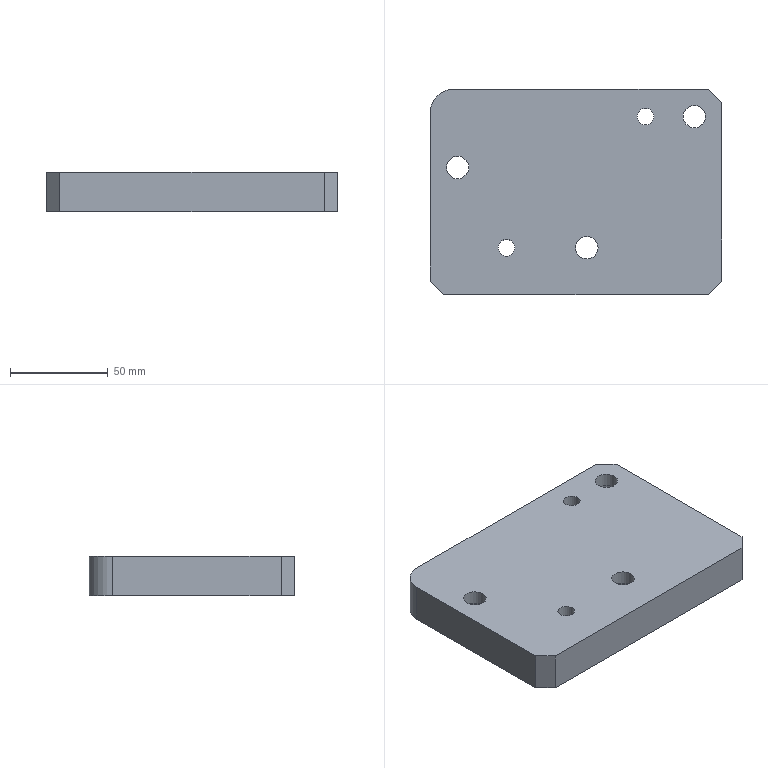Part | STEP file | lll_id606_x_t | 1 solid | 21 faces | box 149 x 105 x 20 mm | volume 296423 mm3 | plane 12 | cylinder 9 | commonest cylinder face diameters 11.509 x3 18.007 x3 8.505 x2 24 x1
STEP:
#1=CARTESIAN_POINT('',(372.248,164.5,2.5));
#2=VERTEX_POINT('',#1);
#3=CARTESIAN_POINT('',(376.5,164.5,2.5));
#4=DIRECTION('',(0.,0.,-1.));
#5=DIRECTION('',(-1.,0.,0.));
#6=AXIS2_PLACEMENT_3D('',#3,#4,#5);
#7=CIRCLE('',#6,4.253);
#8=EDGE_CURVE('',#2,#2,#7,.T.);
#9=ORIENTED_EDGE('',*,*,#8,.F.);
#10=EDGE_LOOP('',(#9));
#11=FACE_BOUND('',#10,.T.);
#12=CARTESIAN_POINT('',(289.504,138.5,2.5));
#13=VERTEX_POINT('',#12);
#14=CARTESIAN_POINT('',(280.5,138.5,2.5));
#15=DIRECTION('',(0.,0.,1.));
#16=DIRECTION('',(1.,0.,0.));
#17=AXIS2_PLACEMENT_3D('',#14,#15,#16);
#18=CIRCLE('',#17,9.004);
#19=EDGE_CURVE('',#13,#13,#18,.T.);
#20=ORIENTED_EDGE('',*,*,#19,.T.);
#21=EDGE_LOOP('',(#20));
#22=FACE_BOUND('',#21,.T.);
#23=CARTESIAN_POINT('',(266.5,166.5,2.5));
#24=VERTEX_POINT('',#23);
#25=CARTESIAN_POINT('',(266.5,80.5,2.5));
#26=VERTEX_POINT('',#25);
#27=CARTESIAN_POINT('',(266.5,130.75,2.5));
#28=DIRECTION('',(0.,-1.,0.));
#29=VECTOR('',#28,1.);
#30=LINE('',#27,#29);
#31=EDGE_CURVE('',#24,#26,#30,.T.);
#32=ORIENTED_EDGE('',*,*,#31,.F.);
#33=CARTESIAN_POINT('',(278.5,178.5,2.5));
#34=VERTEX_POINT('',#33);
#35=CARTESIAN_POINT('',(278.5,166.5,2.5));
#36=DIRECTION('',(0.,0.,-1.));
#37=DIRECTION('',(-1.,0.,0.));
#38=AXIS2_PLACEMENT_3D('',#35,#36,#37);
#39=CIRCLE('',#38,12.);
#40=EDGE_CURVE('',#24,#34,#39,.T.);
#41=ORIENTED_EDGE('',*,*,#40,.T.);
#42=CARTESIAN_POINT('',(408.5,178.5,2.5));
#43=VERTEX_POINT('',#42);
#44=CARTESIAN_POINT('',(437.,178.5,2.5));
#45=DIRECTION('',(-1.,0.,0.));
#46=VECTOR('',#45,1.);
#47=LINE('',#44,#46);
#48=EDGE_CURVE('',#43,#34,#47,.T.);
#49=ORIENTED_EDGE('',*,*,#48,.F.);
#50=CARTESIAN_POINT('',(415.5,171.5,2.5));
#51=VERTEX_POINT('',#50);
#52=CARTESIAN_POINT('',(366.125,220.875,2.5));
#53=DIRECTION('',(-0.7071,0.7071,0.));
#54=VECTOR('',#53,1.);
#55=LINE('',#52,#54);
#56=EDGE_CURVE('',#51,#43,#55,.T.);
#57=ORIENTED_EDGE('',*,*,#56,.F.);
#58=CARTESIAN_POINT('',(415.5,80.5,2.5));
#59=VERTEX_POINT('',#58);
#60=CARTESIAN_POINT('',(415.5,130.75,2.5));
#61=DIRECTION('',(0.,1.,0.));
#62=VECTOR('',#61,1.);
#63=LINE('',#60,#62);
#64=EDGE_CURVE('',#59,#51,#63,.T.);
#65=ORIENTED_EDGE('',*,*,#64,.F.);
#66=CARTESIAN_POINT('',(408.5,73.5,2.5));
#67=VERTEX_POINT('',#66);
#68=CARTESIAN_POINT('',(531.875,196.875,2.5));
#69=DIRECTION('',(0.7071,0.7071,0.));
#70=VECTOR('',#69,1.);
#71=LINE('',#68,#70);
#72=EDGE_CURVE('',#67,#59,#71,.T.);
#73=ORIENTED_EDGE('',*,*,#72,.F.);
#74=CARTESIAN_POINT('',(273.5,73.5,2.5));
#75=VERTEX_POINT('',#74);
#76=CARTESIAN_POINT('',(437.,73.5,2.5));
#77=DIRECTION('',(1.,0.,0.));
#78=VECTOR('',#77,1.);
#79=LINE('',#76,#78);
#80=EDGE_CURVE('',#75,#67,#79,.T.);
#81=ORIENTED_EDGE('',*,*,#80,.F.);
#82=CARTESIAN_POINT('',(246.125,100.875,2.5));
#83=DIRECTION('',(0.7071,-0.7071,0.));
#84=VECTOR('',#83,1.);
#85=LINE('',#82,#84);
#86=EDGE_CURVE('',#26,#75,#85,.T.);
#87=ORIENTED_EDGE('',*,*,#86,.F.);
#88=EDGE_LOOP('',(#32,#41,#49,#57,#65,#73,#81,#87));
#89=FACE_BOUND('',#88,.T.);
#90=CARTESIAN_POINT('',(355.504,97.5,2.5));
#91=VERTEX_POINT('',#90);
#92=CARTESIAN_POINT('',(346.5,97.5,2.5));
#93=DIRECTION('',(0.,0.,1.));
#94=DIRECTION('',(1.,0.,0.));
#95=AXIS2_PLACEMENT_3D('',#92,#93,#94);
#96=CIRCLE('',#95,9.004);
#97=EDGE_CURVE('',#91,#91,#96,.T.);
#98=ORIENTED_EDGE('',*,*,#97,.T.);
#99=EDGE_LOOP('',(#98));
#100=FACE_BOUND('',#99,.T.);
#101=CARTESIAN_POINT('',(301.248,97.5,2.5));
#102=VERTEX_POINT('',#101);
#103=CARTESIAN_POINT('',(305.5,97.5,2.5));
#104=DIRECTION('',(0.,0.,-1.));
#105=DIRECTION('',(-1.,0.,0.));
#106=AXIS2_PLACEMENT_3D('',#103,#104,#105);
#107=CIRCLE('',#106,4.253);
#108=EDGE_CURVE('',#102,#102,#107,.T.);
#109=ORIENTED_EDGE('',*,*,#108,.F.);
#110=EDGE_LOOP('',(#109));
#111=FACE_BOUND('',#110,.T.);
#112=CARTESIAN_POINT('',(410.504,164.5,2.5));
#113=VERTEX_POINT('',#112);
#114=CARTESIAN_POINT('',(401.5,164.5,2.5));
#115=DIRECTION('',(0.,0.,1.));
#116=DIRECTION('',(1.,0.,0.));
#117=AXIS2_PLACEMENT_3D('',#114,#115,#116);
#118=CIRCLE('',#117,9.004);
#119=EDGE_CURVE('',#113,#113,#118,.T.);
#120=ORIENTED_EDGE('',*,*,#119,.T.);
#121=EDGE_LOOP('',(#120));
#122=FACE_BOUND('',#121,.T.);
#123=CARTESIAN_POINT('',(437.,291.75,2.5));
#124=DIRECTION('',(0.,0.,-1.));
#125=DIRECTION('',(1.,0.,0.));
#126=AXIS2_PLACEMENT_3D('',#123,#124,#125);
#127=PLANE('',#126);
#128=ADVANCED_FACE('',(#11,#22,#89,#100,#111,#122),#127,.T.);
#129=CARTESIAN_POINT('',(380.753,164.5,22.5));
#130=VERTEX_POINT('',#129);
#131=CARTESIAN_POINT('',(376.5,164.5,22.5));
#132=DIRECTION('',(0.,0.,1.));
#133=DIRECTION('',(1.,0.,0.));
#134=AXIS2_PLACEMENT_3D('',#131,#132,#133);
#135=CIRCLE('',#134,4.253);
#136=EDGE_CURVE('',#130,#130,#135,.T.);
#137=ORIENTED_EDGE('',*,*,#136,.F.);
#138=EDGE_LOOP('',(#137));
#139=FACE_BOUND('',#138,.T.);
#140=CARTESIAN_POINT('',(407.255,164.5,22.5));
#141=VERTEX_POINT('',#140);
#142=CARTESIAN_POINT('',(401.5,164.5,22.5));
#143=DIRECTION('',(0.,0.,1.));
#144=DIRECTION('',(1.,0.,0.));
#145=AXIS2_PLACEMENT_3D('',#142,#143,#144);
#146=CIRCLE('',#145,5.755);
#147=EDGE_CURVE('',#141,#141,#146,.T.);
#148=ORIENTED_EDGE('',*,*,#147,.F.);
#149=EDGE_LOOP('',(#148));
#150=FACE_BOUND('',#149,.T.);
#151=CARTESIAN_POINT('',(309.753,97.5,22.5));
#152=VERTEX_POINT('',#151);
#153=CARTESIAN_POINT('',(305.5,97.5,22.5));
#154=DIRECTION('',(0.,0.,1.));
#155=DIRECTION('',(1.,0.,0.));
#156=AXIS2_PLACEMENT_3D('',#153,#154,#155);
#157=CIRCLE('',#156,4.253);
#158=EDGE_CURVE('',#152,#152,#157,.T.);
#159=ORIENTED_EDGE('',*,*,#158,.F.);
#160=EDGE_LOOP('',(#159));
#161=FACE_BOUND('',#160,.T.);
#162=CARTESIAN_POINT('',(286.255,138.5,22.5));
#163=VERTEX_POINT('',#162);
#164=CARTESIAN_POINT('',(280.5,138.5,22.5));
#165=DIRECTION('',(0.,0.,1.));
#166=DIRECTION('',(1.,0.,0.));
#167=AXIS2_PLACEMENT_3D('',#164,#165,#166);
#168=CIRCLE('',#167,5.755);
#169=EDGE_CURVE('',#163,#163,#168,.T.);
#170=ORIENTED_EDGE('',*,*,#169,.F.);
#171=EDGE_LOOP('',(#170));
#172=FACE_BOUND('',#171,.T.);
#173=CARTESIAN_POINT('',(352.255,97.5,22.5));
#174=VERTEX_POINT('',#173);
#175=CARTESIAN_POINT('',(346.5,97.5,22.5));
#176=DIRECTION('',(0.,0.,1.));
#177=DIRECTION('',(1.,0.,0.));
#178=AXIS2_PLACEMENT_3D('',#175,#176,#177);
#179=CIRCLE('',#178,5.755);
#180=EDGE_CURVE('',#174,#174,#179,.T.);
#181=ORIENTED_EDGE('',*,*,#180,.F.);
#182=EDGE_LOOP('',(#181));
#183=FACE_BOUND('',#182,.T.);
#184=CARTESIAN_POINT('',(278.5,178.5,22.5));
#185=VERTEX_POINT('',#184);
#186=CARTESIAN_POINT('',(408.5,178.5,22.5));
#187=VERTEX_POINT('',#186);
#188=CARTESIAN_POINT('',(437.,178.5,22.5));
#189=DIRECTION('',(1.,0.,0.));
#190=VECTOR('',#189,1.);
#191=LINE('',#188,#190);
#192=EDGE_CURVE('',#185,#187,#191,.T.);
#193=ORIENTED_EDGE('',*,*,#192,.F.);
#194=CARTESIAN_POINT('',(266.5,166.5,22.5));
#195=VERTEX_POINT('',#194);
#196=CARTESIAN_POINT('',(278.5,166.5,22.5));
#197=DIRECTION('',(0.,0.,1.));
#198=DIRECTION('',(1.,0.,0.));
#199=AXIS2_PLACEMENT_3D('',#196,#197,#198);
#200=CIRCLE('',#199,12.);
#201=EDGE_CURVE('',#185,#195,#200,.T.);
#202=ORIENTED_EDGE('',*,*,#201,.T.);
#203=CARTESIAN_POINT('',(266.5,80.5,22.5));
#204=VERTEX_POINT('',#203);
#205=CARTESIAN_POINT('',(266.5,130.75,22.5));
#206=DIRECTION('',(0.,1.,0.));
#207=VECTOR('',#206,1.);
#208=LINE('',#205,#207);
#209=EDGE_CURVE('',#204,#195,#208,.T.);
#210=ORIENTED_EDGE('',*,*,#209,.F.);
#211=CARTESIAN_POINT('',(273.5,73.5,22.5));
#212=VERTEX_POINT('',#211);
#213=CARTESIAN_POINT('',(246.125,100.875,22.5));
#214=DIRECTION('',(-0.7071,0.7071,0.));
#215=VECTOR('',#214,1.);
#216=LINE('',#213,#215);
#217=EDGE_CURVE('',#212,#204,#216,.T.);
#218=ORIENTED_EDGE('',*,*,#217,.F.);
#219=CARTESIAN_POINT('',(408.5,73.5,22.5));
#220=VERTEX_POINT('',#219);
#221=CARTESIAN_POINT('',(437.,73.5,22.5));
#222=DIRECTION('',(-1.,0.,0.));
#223=VECTOR('',#222,1.);
#224=LINE('',#221,#223);
#225=EDGE_CURVE('',#220,#212,#224,.T.);
#226=ORIENTED_EDGE('',*,*,#225,.F.);
#227=CARTESIAN_POINT('',(415.5,80.5,22.5));
#228=VERTEX_POINT('',#227);
#229=CARTESIAN_POINT('',(531.875,196.875,22.5));
#230=DIRECTION('',(-0.7071,-0.7071,0.));
#231=VECTOR('',#230,1.);
#232=LINE('',#229,#231);
#233=EDGE_CURVE('',#228,#220,#232,.T.);
#234=ORIENTED_EDGE('',*,*,#233,.F.);
#235=CARTESIAN_POINT('',(415.5,171.5,22.5));
#236=VERTEX_POINT('',#235);
#237=CARTESIAN_POINT('',(415.5,130.75,22.5));
#238=DIRECTION('',(0.,-1.,0.));
#239=VECTOR('',#238,1.);
#240=LINE('',#237,#239);
#241=EDGE_CURVE('',#236,#228,#240,.T.);
#242=ORIENTED_EDGE('',*,*,#241,.F.);
#243=CARTESIAN_POINT('',(366.125,220.875,22.5));
#244=DIRECTION('',(0.7071,-0.7071,0.));
#245=VECTOR('',#244,1.);
#246=LINE('',#243,#245);
#247=EDGE_CURVE('',#187,#236,#246,.T.);
#248=ORIENTED_EDGE('',*,*,#247,.F.);
#249=EDGE_LOOP('',(#193,#202,#210,#218,#226,#234,#242,#248));
#250=FACE_BOUND('',#249,.T.);
#251=CARTESIAN_POINT('',(437.,291.75,22.5));
#252=DIRECTION('',(0.,0.,1.));
#253=DIRECTION('',(-1.,0.,0.));
#254=AXIS2_PLACEMENT_3D('',#251,#252,#253);
#255=PLANE('',#254);
#256=ADVANCED_FACE('',(#139,#150,#161,#172,#183,#250),#255,.T.);
#257=ORIENTED_EDGE('',*,*,#241,.T.);
#258=CARTESIAN_POINT('',(415.5,80.5,-10.15));
#259=DIRECTION('',(0.,0.,1.));
#260=VECTOR('',#259,1.);
#261=LINE('',#258,#260);
#262=EDGE_CURVE('',#59,#228,#261,.T.);
#263=ORIENTED_EDGE('',*,*,#262,.F.);
#264=ORIENTED_EDGE('',*,*,#64,.T.);
#265=CARTESIAN_POINT('',(415.5,171.5,2.5));
#266=DIRECTION('',(0.,0.,-1.));
#267=VECTOR('',#266,1.);
#268=LINE('',#265,#267);
#269=EDGE_CURVE('',#236,#51,#268,.T.);
#270=ORIENTED_EDGE('',*,*,#269,.F.);
#271=EDGE_LOOP('',(#257,#263,#264,#270));
#272=FACE_OUTER_BOUND('',#271,.T.);
#273=CARTESIAN_POINT('',(415.5,130.75,-10.15));
#274=DIRECTION('',(1.,0.,0.));
#275=DIRECTION('',(0.,0.,-1.));
#276=AXIS2_PLACEMENT_3D('',#273,#274,#275);
#277=PLANE('',#276);
#278=ADVANCED_FACE('',(#272),#277,.T.);
#279=ORIENTED_EDGE('',*,*,#225,.T.);
#280=CARTESIAN_POINT('',(273.5,73.5,-10.15));
#281=DIRECTION('',(0.,0.,1.));
#282=VECTOR('',#281,1.);
#283=LINE('',#280,#282);
#284=EDGE_CURVE('',#75,#212,#283,.T.);
#285=ORIENTED_EDGE('',*,*,#284,.F.);
#286=ORIENTED_EDGE('',*,*,#80,.T.);
#287=CARTESIAN_POINT('',(408.5,73.5,-10.15));
#288=DIRECTION('',(0.,0.,-1.));
#289=VECTOR('',#288,1.);
#290=LINE('',#287,#289);
#291=EDGE_CURVE('',#220,#67,#290,.T.);
#292=ORIENTED_EDGE('',*,*,#291,.F.);
#293=EDGE_LOOP('',(#279,#285,#286,#292));
#294=FACE_OUTER_BOUND('',#293,.T.);
#295=CARTESIAN_POINT('',(337.5,73.5,-10.15));
#296=DIRECTION('',(0.,-1.,0.));
#297=DIRECTION('',(0.,0.,-1.));
#298=AXIS2_PLACEMENT_3D('',#295,#296,#297);
#299=PLANE('',#298);
#300=ADVANCED_FACE('',(#294),#299,.T.);
#301=ORIENTED_EDGE('',*,*,#209,.T.);
#302=CARTESIAN_POINT('',(266.5,166.5,-10.15));
#303=DIRECTION('',(0.,0.,-1.));
#304=VECTOR('',#303,1.);
#305=LINE('',#302,#304);
#306=EDGE_CURVE('',#195,#24,#305,.T.);
#307=ORIENTED_EDGE('',*,*,#306,.T.);
#308=ORIENTED_EDGE('',*,*,#31,.T.);
#309=CARTESIAN_POINT('',(266.5,80.5,-10.15));
#310=DIRECTION('',(0.,0.,-1.));
#311=VECTOR('',#310,1.);
#312=LINE('',#309,#311);
#313=EDGE_CURVE('',#204,#26,#312,.T.);
#314=ORIENTED_EDGE('',*,*,#313,.F.);
#315=EDGE_LOOP('',(#301,#307,#308,#314));
#316=FACE_OUTER_BOUND('',#315,.T.);
#317=CARTESIAN_POINT('',(266.5,130.75,-10.15));
#318=DIRECTION('',(-1.,0.,0.));
#319=DIRECTION('',(0.,0.,1.));
#320=AXIS2_PLACEMENT_3D('',#317,#318,#319);
#321=PLANE('',#320);
#322=ADVANCED_FACE('',(#316),#321,.T.);
#323=ORIENTED_EDGE('',*,*,#48,.T.);
#324=CARTESIAN_POINT('',(278.5,178.5,-10.15));
#325=DIRECTION('',(0.,0.,1.));
#326=VECTOR('',#325,1.);
#327=LINE('',#324,#326);
#328=EDGE_CURVE('',#34,#185,#327,.T.);
#329=ORIENTED_EDGE('',*,*,#328,.T.);
#330=ORIENTED_EDGE('',*,*,#192,.T.);
#331=CARTESIAN_POINT('',(408.5,178.5,22.5));
#332=DIRECTION('',(0.,0.,1.));
#333=VECTOR('',#332,1.);
#334=LINE('',#331,#333);
#335=EDGE_CURVE('',#43,#187,#334,.T.);
#336=ORIENTED_EDGE('',*,*,#335,.F.);
#337=EDGE_LOOP('',(#323,#329,#330,#336));
#338=FACE_OUTER_BOUND('',#337,.T.);
#339=CARTESIAN_POINT('',(350.,178.5,12.5));
#340=DIRECTION('',(0.,-1.,0.));
#341=DIRECTION('',(0.,0.,-1.));
#342=AXIS2_PLACEMENT_3D('',#339,#340,#341);
#343=PLANE('',#342);
#344=ADVANCED_FACE('',(#338),#343,.F.);
#345=ORIENTED_EDGE('',*,*,#180,.T.);
#346=EDGE_LOOP('',(#345));
#347=FACE_BOUND('',#346,.T.);
#348=CARTESIAN_POINT('',(352.255,97.5,15.5));
#349=VERTEX_POINT('',#348);
#350=CARTESIAN_POINT('',(346.5,97.5,15.5));
#351=DIRECTION('',(0.,0.,1.));
#352=DIRECTION('',(1.,0.,0.));
#353=AXIS2_PLACEMENT_3D('',#350,#351,#352);
#354=CIRCLE('',#353,5.755);
#355=EDGE_CURVE('',#349,#349,#354,.T.);
#356=ORIENTED_EDGE('',*,*,#355,.F.);
#357=EDGE_LOOP('',(#356));
#358=FACE_BOUND('',#357,.T.);
#359=CARTESIAN_POINT('',(346.5,97.5,-2.5));
#360=DIRECTION('',(0.,0.,1.));
#361=DIRECTION('',(1.,0.,0.));
#362=AXIS2_PLACEMENT_3D('',#359,#360,#361);
#363=CYLINDRICAL_SURFACE('',#362,5.755);
#364=ADVANCED_FACE('',(#347,#358),#363,.F.);
#365=ORIENTED_EDGE('',*,*,#355,.T.);
#366=EDGE_LOOP('',(#365));
#367=FACE_BOUND('',#366,.T.);
#368=CARTESIAN_POINT('',(355.504,97.5,15.5));
#369=VERTEX_POINT('',#368);
#370=CARTESIAN_POINT('',(346.5,97.5,15.5));
#371=DIRECTION('',(0.,0.,1.));
#372=DIRECTION('',(1.,0.,0.));
#373=AXIS2_PLACEMENT_3D('',#370,#371,#372);
#374=CIRCLE('',#373,9.004);
#375=EDGE_CURVE('',#369,#369,#374,.T.);
#376=ORIENTED_EDGE('',*,*,#375,.F.);
#377=EDGE_LOOP('',(#376));
#378=FACE_BOUND('',#377,.T.);
#379=CARTESIAN_POINT('',(346.5,97.5,15.5));
#380=DIRECTION('',(0.,0.,1.));
#381=DIRECTION('',(1.,0.,0.));
#382=AXIS2_PLACEMENT_3D('',#379,#380,#381);
#383=PLANE('',#382);
#384=ADVANCED_FACE('',(#367,#378),#383,.F.);
#385=ORIENTED_EDGE('',*,*,#375,.T.);
#386=EDGE_LOOP('',(#385));
#387=FACE_BOUND('',#386,.T.);
#388=ORIENTED_EDGE('',*,*,#97,.F.);
#389=EDGE_LOOP('',(#388));
#390=FACE_BOUND('',#389,.T.);
#391=CARTESIAN_POINT('',(346.5,97.5,2.5));
#392=DIRECTION('',(0.,0.,1.));
#393=DIRECTION('',(1.,0.,0.));
#394=AXIS2_PLACEMENT_3D('',#391,#392,#393);
#395=CYLINDRICAL_SURFACE('',#394,9.004);
#396=ADVANCED_FACE('',(#387,#390),#395,.F.);
#397=ORIENTED_EDGE('',*,*,#169,.T.);
#398=EDGE_LOOP('',(#397));
#399=FACE_BOUND('',#398,.T.);
#400=CARTESIAN_POINT('',(286.255,138.5,15.5));
#401=VERTEX_POINT('',#400);
#402=CARTESIAN_POINT('',(280.5,138.5,15.5));
#403=DIRECTION('',(0.,0.,1.));
#404=DIRECTION('',(1.,0.,0.));
#405=AXIS2_PLACEMENT_3D('',#402,#403,#404);
#406=CIRCLE('',#405,5.755);
#407=EDGE_CURVE('',#401,#401,#406,.T.);
#408=ORIENTED_EDGE('',*,*,#407,.F.);
#409=EDGE_LOOP('',(#408));
#410=FACE_BOUND('',#409,.T.);
#411=CARTESIAN_POINT('',(280.5,138.5,-2.5));
#412=DIRECTION('',(0.,0.,1.));
#413=DIRECTION('',(1.,0.,0.));
#414=AXIS2_PLACEMENT_3D('',#411,#412,#413);
#415=CYLINDRICAL_SURFACE('',#414,5.755);
#416=ADVANCED_FACE('',(#399,#410),#415,.F.);
#417=ORIENTED_EDGE('',*,*,#407,.T.);
#418=EDGE_LOOP('',(#417));
#419=FACE_BOUND('',#418,.T.);
#420=CARTESIAN_POINT('',(289.504,138.5,15.5));
#421=VERTEX_POINT('',#420);
#422=CARTESIAN_POINT('',(280.5,138.5,15.5));
#423=DIRECTION('',(0.,0.,1.));
#424=DIRECTION('',(1.,0.,0.));
#425=AXIS2_PLACEMENT_3D('',#422,#423,#424);
#426=CIRCLE('',#425,9.004);
#427=EDGE_CURVE('',#421,#421,#426,.T.);
#428=ORIENTED_EDGE('',*,*,#427,.F.);
#429=EDGE_LOOP('',(#428));
#430=FACE_BOUND('',#429,.T.);
#431=CARTESIAN_POINT('',(280.5,138.5,15.5));
#432=DIRECTION('',(0.,0.,1.));
#433=DIRECTION('',(1.,0.,0.));
#434=AXIS2_PLACEMENT_3D('',#431,#432,#433);
#435=PLANE('',#434);
#436=ADVANCED_FACE('',(#419,#430),#435,.F.);
#437=ORIENTED_EDGE('',*,*,#427,.T.);
#438=EDGE_LOOP('',(#437));
#439=FACE_BOUND('',#438,.T.);
#440=ORIENTED_EDGE('',*,*,#19,.F.);
#441=EDGE_LOOP('',(#440));
#442=FACE_BOUND('',#441,.T.);
#443=CARTESIAN_POINT('',(280.5,138.5,2.5));
#444=DIRECTION('',(0.,0.,1.));
#445=DIRECTION('',(1.,0.,0.));
#446=AXIS2_PLACEMENT_3D('',#443,#444,#445);
#447=CYLINDRICAL_SURFACE('',#446,9.004);
#448=ADVANCED_FACE('',(#439,#442),#447,.F.);
#449=ORIENTED_EDGE('',*,*,#108,.T.);
#450=EDGE_LOOP('',(#449));
#451=FACE_BOUND('',#450,.T.);
#452=ORIENTED_EDGE('',*,*,#158,.T.);
#453=EDGE_LOOP('',(#452));
#454=FACE_BOUND('',#453,.T.);
#455=CARTESIAN_POINT('',(305.5,97.5,-2.5));
#456=DIRECTION('',(0.,0.,1.));
#457=DIRECTION('',(1.,0.,0.));
#458=AXIS2_PLACEMENT_3D('',#455,#456,#457);
#459=CYLINDRICAL_SURFACE('',#458,4.253);
#460=ADVANCED_FACE('',(#451,#454),#459,.F.);
#461=ORIENTED_EDGE('',*,*,#147,.T.);
#462=EDGE_LOOP('',(#461));
#463=FACE_BOUND('',#462,.T.);
#464=CARTESIAN_POINT('',(407.255,164.5,15.5));
#465=VERTEX_POINT('',#464);
#466=CARTESIAN_POINT('',(401.5,164.5,15.5));
#467=DIRECTION('',(0.,0.,1.));
#468=DIRECTION('',(1.,0.,0.));
#469=AXIS2_PLACEMENT_3D('',#466,#467,#468);
#470=CIRCLE('',#469,5.755);
#471=EDGE_CURVE('',#465,#465,#470,.T.);
#472=ORIENTED_EDGE('',*,*,#471,.F.);
#473=EDGE_LOOP('',(#472));
#474=FACE_BOUND('',#473,.T.);
#475=CARTESIAN_POINT('',(401.5,164.5,-2.5));
#476=DIRECTION('',(0.,0.,1.));
#477=DIRECTION('',(1.,0.,0.));
#478=AXIS2_PLACEMENT_3D('',#475,#476,#477);
#479=CYLINDRICAL_SURFACE('',#478,5.755);
#480=ADVANCED_FACE('',(#463,#474),#479,.F.);
#481=ORIENTED_EDGE('',*,*,#471,.T.);
#482=EDGE_LOOP('',(#481));
#483=FACE_BOUND('',#482,.T.);
#484=CARTESIAN_POINT('',(410.504,164.5,15.5));
#485=VERTEX_POINT('',#484);
#486=CARTESIAN_POINT('',(401.5,164.5,15.5));
#487=DIRECTION('',(0.,0.,1.));
#488=DIRECTION('',(1.,0.,0.));
#489=AXIS2_PLACEMENT_3D('',#486,#487,#488);
#490=CIRCLE('',#489,9.004);
#491=EDGE_CURVE('',#485,#485,#490,.T.);
#492=ORIENTED_EDGE('',*,*,#491,.F.);
#493=EDGE_LOOP('',(#492));
#494=FACE_BOUND('',#493,.T.);
#495=CARTESIAN_POINT('',(401.5,164.5,15.5));
#496=DIRECTION('',(0.,0.,1.));
#497=DIRECTION('',(1.,0.,0.));
#498=AXIS2_PLACEMENT_3D('',#495,#496,#497);
#499=PLANE('',#498);
#500=ADVANCED_FACE('',(#483,#494),#499,.F.);
#501=ORIENTED_EDGE('',*,*,#491,.T.);
#502=EDGE_LOOP('',(#501));
#503=FACE_BOUND('',#502,.T.);
#504=ORIENTED_EDGE('',*,*,#119,.F.);
#505=EDGE_LOOP('',(#504));
#506=FACE_BOUND('',#505,.T.);
#507=CARTESIAN_POINT('',(401.5,164.5,2.5));
#508=DIRECTION('',(0.,0.,1.));
#509=DIRECTION('',(1.,0.,0.));
#510=AXIS2_PLACEMENT_3D('',#507,#508,#509);
#511=CYLINDRICAL_SURFACE('',#510,9.004);
#512=ADVANCED_FACE('',(#503,#506),#511,.F.);
#513=ORIENTED_EDGE('',*,*,#8,.T.);
#514=EDGE_LOOP('',(#513));
#515=FACE_BOUND('',#514,.T.);
#516=ORIENTED_EDGE('',*,*,#136,.T.);
#517=EDGE_LOOP('',(#516));
#518=FACE_BOUND('',#517,.T.);
#519=CARTESIAN_POINT('',(376.5,164.5,-2.5));
#520=DIRECTION('',(0.,0.,1.));
#521=DIRECTION('',(1.,0.,0.));
#522=AXIS2_PLACEMENT_3D('',#519,#520,#521);
#523=CYLINDRICAL_SURFACE('',#522,4.253);
#524=ADVANCED_FACE('',(#515,#518),#523,.F.);
#525=ORIENTED_EDGE('',*,*,#56,.T.);
#526=ORIENTED_EDGE('',*,*,#335,.T.);
#527=ORIENTED_EDGE('',*,*,#247,.T.);
#528=ORIENTED_EDGE('',*,*,#269,.T.);
#529=EDGE_LOOP('',(#525,#526,#527,#528));
#530=FACE_OUTER_BOUND('',#529,.T.);
#531=CARTESIAN_POINT('',(408.5,178.5,12.5));
#532=DIRECTION('',(0.7071,0.7071,0.));
#533=DIRECTION('',(0.,0.,1.));
#534=AXIS2_PLACEMENT_3D('',#531,#532,#533);
#535=PLANE('',#534);
#536=ADVANCED_FACE('',(#530),#535,.T.);
#537=ORIENTED_EDGE('',*,*,#72,.T.);
#538=ORIENTED_EDGE('',*,*,#262,.T.);
#539=ORIENTED_EDGE('',*,*,#233,.T.);
#540=ORIENTED_EDGE('',*,*,#291,.T.);
#541=EDGE_LOOP('',(#537,#538,#539,#540));
#542=FACE_OUTER_BOUND('',#541,.T.);
#543=CARTESIAN_POINT('',(415.5,80.5,-10.15));
#544=DIRECTION('',(-0.7071,0.7071,0.));
#545=DIRECTION('',(0.,0.,-1.));
#546=AXIS2_PLACEMENT_3D('',#543,#544,#545);
#547=PLANE('',#546);
#548=ADVANCED_FACE('',(#542),#547,.F.);
#549=ORIENTED_EDGE('',*,*,#86,.T.);
#550=ORIENTED_EDGE('',*,*,#284,.T.);
#551=ORIENTED_EDGE('',*,*,#217,.T.);
#552=ORIENTED_EDGE('',*,*,#313,.T.);
#553=EDGE_LOOP('',(#549,#550,#551,#552));
#554=FACE_OUTER_BOUND('',#553,.T.);
#555=CARTESIAN_POINT('',(273.5,73.5,-10.15));
#556=DIRECTION('',(0.7071,0.7071,0.));
#557=DIRECTION('',(0.,0.,-1.));
#558=AXIS2_PLACEMENT_3D('',#555,#556,#557);
#559=PLANE('',#558);
#560=ADVANCED_FACE('',(#554),#559,.F.);
#561=ORIENTED_EDGE('',*,*,#40,.F.);
#562=ORIENTED_EDGE('',*,*,#306,.F.);
#563=ORIENTED_EDGE('',*,*,#201,.F.);
#564=ORIENTED_EDGE('',*,*,#328,.F.);
#565=EDGE_LOOP('',(#561,#562,#563,#564));
#566=FACE_OUTER_BOUND('',#565,.T.);
#567=CARTESIAN_POINT('',(278.5,166.5,-10.15));
#568=DIRECTION('',(0.,0.,1.));
#569=DIRECTION('',(-1.,0.,0.));
#570=AXIS2_PLACEMENT_3D('',#567,#568,#569);
#571=CYLINDRICAL_SURFACE('',#570,12.);
#572=ADVANCED_FACE('',(#566),#571,.T.);
#573=CLOSED_SHELL('',(#128,#256,#278,#300,#322,#344,#364,#384,#396,#416,#436,#448,#460,#480,#500,#512,#524,#536,#548,#560,#572));
#574=MANIFOLD_SOLID_BREP('',#573);
#575=(LENGTH_UNIT()NAMED_UNIT(*)SI_UNIT(.MILLI.,.METRE.));
#576=UNCERTAINTY_MEASURE_WITH_UNIT(LENGTH_MEASURE(0.00002),#575,'','');
#577=(NAMED_UNIT(*)PLANE_ANGLE_UNIT()SI_UNIT($,.RADIAN.));
#578=PLANE_ANGLE_MEASURE_WITH_UNIT(PLANE_ANGLE_MEASURE(0.01745),#577);
#579=DIMENSIONAL_EXPONENTS(0.,0.,0.,0.,0.,0.,0.);
#580=(CONVERSION_BASED_UNIT('DEGREE',#578)NAMED_UNIT(#579)PLANE_ANGLE_UNIT());
#581=(NAMED_UNIT(*)SI_UNIT($,.STERADIAN.)SOLID_ANGLE_UNIT());
#582=(GEOMETRIC_REPRESENTATION_CONTEXT(3)GLOBAL_UNCERTAINTY_ASSIGNED_CONTEXT((#576))GLOBAL_UNIT_ASSIGNED_CONTEXT((#575,#580,#581))REPRESENTATION_CONTEXT('',''));
#583=ADVANCED_BREP_SHAPE_REPRESENTATION('',(#574),#582);